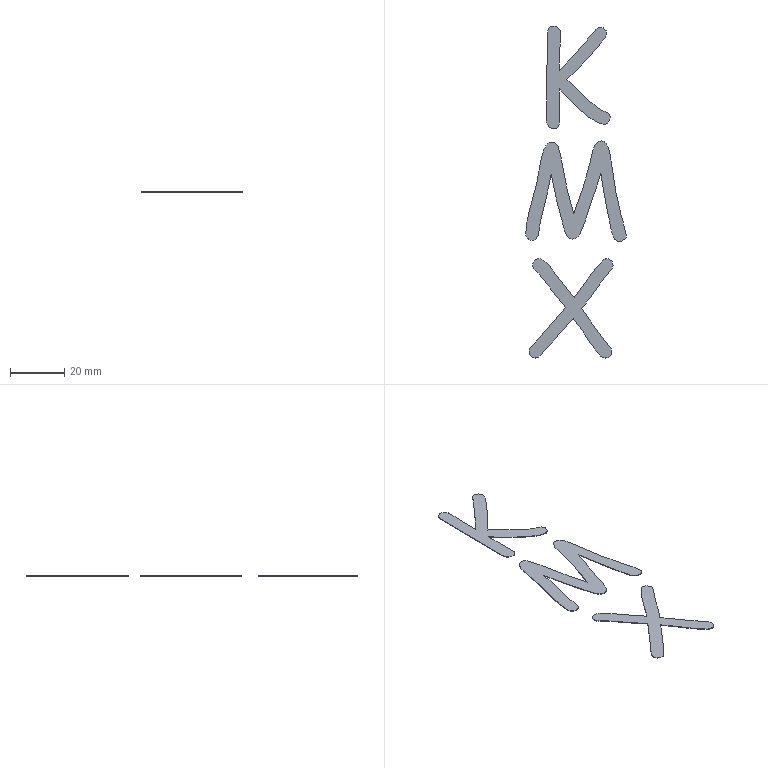Part | STEP file | KMX Label | 3 solids | 95 faces | box 37.188 x 122.835 x 0.2 mm | volume 278.428 mm3 | spline 65 | plane 30